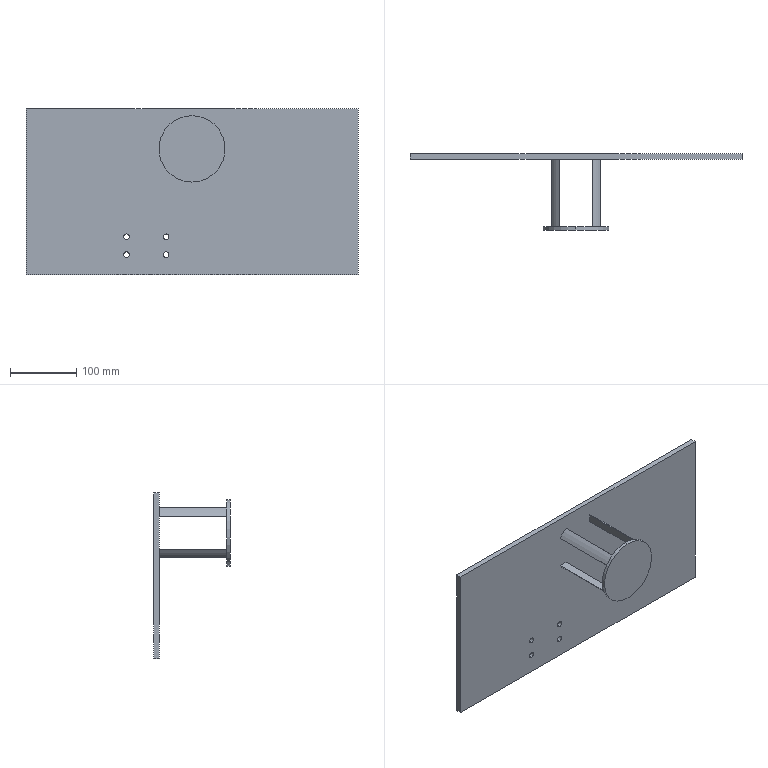Part | SolidWorks | features BaseBody 1 | 1 solid | 30 faces | box 500 x 114.889 x 250 mm | volume 1072983 mm3 | plane 16 | cylinder 14 | commonest cylinder face diameters 8.55 x8 90 x4 100 x2
STEP:
#1=CARTESIAN_POINT('',(211.045,8.,61.824));
#2=VERTEX_POINT('',#1);
#3=CARTESIAN_POINT('',(211.045,8.,53.274));
#4=VERTEX_POINT('',#3);
#5=CARTESIAN_POINT('',(211.045,8.,57.549));
#6=DIRECTION('',(0.,-1.,0.));
#7=DIRECTION('',(0.,0.,-1.));
#8=AXIS2_PLACEMENT_3D('',#5,#6,#7);
#9=CIRCLE('',#8,4.275);
#10=EDGE_CURVE('',#2,#4,#9,.T.);
#11=ORIENTED_EDGE('',*,*,#10,.F.);
#12=CARTESIAN_POINT('',(211.045,0.,61.824));
#13=VERTEX_POINT('',#12);
#14=CARTESIAN_POINT('',(211.045,8.,61.824));
#15=DIRECTION('',(0.,-1.,0.));
#16=VECTOR('',#15,1000.);
#17=LINE('',#14,#16);
#18=EDGE_CURVE('',#2,#13,#17,.T.);
#19=ORIENTED_EDGE('',*,*,#18,.T.);
#20=CARTESIAN_POINT('',(211.045,0.,53.274));
#21=VERTEX_POINT('',#20);
#22=CARTESIAN_POINT('',(211.045,0.,57.549));
#23=DIRECTION('',(0.,1.,0.));
#24=DIRECTION('',(0.,0.,-1.));
#25=AXIS2_PLACEMENT_3D('',#22,#23,#24);
#26=CIRCLE('',#25,4.275);
#27=EDGE_CURVE('',#21,#13,#26,.T.);
#28=ORIENTED_EDGE('',*,*,#27,.F.);
#29=CARTESIAN_POINT('',(211.045,8.,53.274));
#30=DIRECTION('',(0.,-1.,0.));
#31=VECTOR('',#30,1000.);
#32=LINE('',#29,#31);
#33=EDGE_CURVE('',#4,#21,#32,.T.);
#34=ORIENTED_EDGE('',*,*,#33,.F.);
#35=EDGE_LOOP('',(#11,#19,#28,#34));
#36=FACE_OUTER_BOUND('',#35,.T.);
#37=CARTESIAN_POINT('',(211.045,8.,57.549));
#38=DIRECTION('',(0.,-1.,0.));
#39=DIRECTION('',(0.,0.,-1.));
#40=AXIS2_PLACEMENT_3D('',#37,#38,#39);
#41=CYLINDRICAL_SURFACE('',#40,4.275);
#42=ADVANCED_FACE('',(#36),#41,.F.);
#43=CARTESIAN_POINT('',(211.045,8.,34.804));
#44=VERTEX_POINT('',#43);
#45=CARTESIAN_POINT('',(211.045,8.,26.254));
#46=VERTEX_POINT('',#45);
#47=CARTESIAN_POINT('',(211.045,8.,30.529));
#48=DIRECTION('',(0.,-1.,0.));
#49=DIRECTION('',(0.,0.,-1.));
#50=AXIS2_PLACEMENT_3D('',#47,#48,#49);
#51=CIRCLE('',#50,4.275);
#52=EDGE_CURVE('',#44,#46,#51,.T.);
#53=ORIENTED_EDGE('',*,*,#52,.F.);
#54=CARTESIAN_POINT('',(211.045,0.,34.804));
#55=VERTEX_POINT('',#54);
#56=CARTESIAN_POINT('',(211.045,8.,34.804));
#57=DIRECTION('',(0.,-1.,0.));
#58=VECTOR('',#57,1000.);
#59=LINE('',#56,#58);
#60=EDGE_CURVE('',#44,#55,#59,.T.);
#61=ORIENTED_EDGE('',*,*,#60,.T.);
#62=CARTESIAN_POINT('',(211.045,0.,26.254));
#63=VERTEX_POINT('',#62);
#64=CARTESIAN_POINT('',(211.045,0.,30.529));
#65=DIRECTION('',(0.,1.,0.));
#66=DIRECTION('',(0.,0.,-1.));
#67=AXIS2_PLACEMENT_3D('',#64,#65,#66);
#68=CIRCLE('',#67,4.275);
#69=EDGE_CURVE('',#63,#55,#68,.T.);
#70=ORIENTED_EDGE('',*,*,#69,.F.);
#71=CARTESIAN_POINT('',(211.045,8.,26.254));
#72=DIRECTION('',(0.,-1.,0.));
#73=VECTOR('',#72,1000.);
#74=LINE('',#71,#73);
#75=EDGE_CURVE('',#46,#63,#74,.T.);
#76=ORIENTED_EDGE('',*,*,#75,.F.);
#77=EDGE_LOOP('',(#53,#61,#70,#76));
#78=FACE_OUTER_BOUND('',#77,.T.);
#79=CARTESIAN_POINT('',(211.045,8.,30.529));
#80=DIRECTION('',(0.,-1.,0.));
#81=DIRECTION('',(0.,0.,-1.));
#82=AXIS2_PLACEMENT_3D('',#79,#80,#81);
#83=CYLINDRICAL_SURFACE('',#82,4.275);
#84=ADVANCED_FACE('',(#78),#83,.F.);
#85=CARTESIAN_POINT('',(151.435,8.,34.804));
#86=VERTEX_POINT('',#85);
#87=CARTESIAN_POINT('',(151.435,8.,26.254));
#88=VERTEX_POINT('',#87);
#89=CARTESIAN_POINT('',(151.435,8.,30.529));
#90=DIRECTION('',(0.,-1.,0.));
#91=DIRECTION('',(0.,0.,-1.));
#92=AXIS2_PLACEMENT_3D('',#89,#90,#91);
#93=CIRCLE('',#92,4.275);
#94=EDGE_CURVE('',#86,#88,#93,.T.);
#95=ORIENTED_EDGE('',*,*,#94,.F.);
#96=CARTESIAN_POINT('',(151.435,0.,34.804));
#97=VERTEX_POINT('',#96);
#98=CARTESIAN_POINT('',(151.435,8.,34.804));
#99=DIRECTION('',(0.,-1.,0.));
#100=VECTOR('',#99,1000.);
#101=LINE('',#98,#100);
#102=EDGE_CURVE('',#86,#97,#101,.T.);
#103=ORIENTED_EDGE('',*,*,#102,.T.);
#104=CARTESIAN_POINT('',(151.435,0.,26.254));
#105=VERTEX_POINT('',#104);
#106=CARTESIAN_POINT('',(151.435,0.,30.529));
#107=DIRECTION('',(0.,1.,0.));
#108=DIRECTION('',(0.,0.,-1.));
#109=AXIS2_PLACEMENT_3D('',#106,#107,#108);
#110=CIRCLE('',#109,4.275);
#111=EDGE_CURVE('',#105,#97,#110,.T.);
#112=ORIENTED_EDGE('',*,*,#111,.F.);
#113=CARTESIAN_POINT('',(151.435,8.,26.254));
#114=DIRECTION('',(0.,-1.,0.));
#115=VECTOR('',#114,1000.);
#116=LINE('',#113,#115);
#117=EDGE_CURVE('',#88,#105,#116,.T.);
#118=ORIENTED_EDGE('',*,*,#117,.F.);
#119=EDGE_LOOP('',(#95,#103,#112,#118));
#120=FACE_OUTER_BOUND('',#119,.T.);
#121=CARTESIAN_POINT('',(151.435,8.,30.529));
#122=DIRECTION('',(0.,-1.,0.));
#123=DIRECTION('',(0.,0.,-1.));
#124=AXIS2_PLACEMENT_3D('',#121,#122,#123);
#125=CYLINDRICAL_SURFACE('',#124,4.275);
#126=ADVANCED_FACE('',(#120),#125,.F.);
#127=CARTESIAN_POINT('',(151.435,8.,61.824));
#128=VERTEX_POINT('',#127);
#129=CARTESIAN_POINT('',(151.435,8.,53.274));
#130=VERTEX_POINT('',#129);
#131=CARTESIAN_POINT('',(151.435,8.,57.549));
#132=DIRECTION('',(0.,-1.,0.));
#133=DIRECTION('',(0.,0.,-1.));
#134=AXIS2_PLACEMENT_3D('',#131,#132,#133);
#135=CIRCLE('',#134,4.275);
#136=EDGE_CURVE('',#128,#130,#135,.T.);
#137=ORIENTED_EDGE('',*,*,#136,.F.);
#138=CARTESIAN_POINT('',(151.435,0.,61.824));
#139=VERTEX_POINT('',#138);
#140=CARTESIAN_POINT('',(151.435,8.,61.824));
#141=DIRECTION('',(0.,-1.,0.));
#142=VECTOR('',#141,1000.);
#143=LINE('',#140,#142);
#144=EDGE_CURVE('',#128,#139,#143,.T.);
#145=ORIENTED_EDGE('',*,*,#144,.T.);
#146=CARTESIAN_POINT('',(151.435,0.,53.274));
#147=VERTEX_POINT('',#146);
#148=CARTESIAN_POINT('',(151.435,0.,57.549));
#149=DIRECTION('',(0.,1.,0.));
#150=DIRECTION('',(0.,0.,-1.));
#151=AXIS2_PLACEMENT_3D('',#148,#149,#150);
#152=CIRCLE('',#151,4.275);
#153=EDGE_CURVE('',#147,#139,#152,.T.);
#154=ORIENTED_EDGE('',*,*,#153,.F.);
#155=CARTESIAN_POINT('',(151.435,8.,53.274));
#156=DIRECTION('',(0.,-1.,0.));
#157=VECTOR('',#156,1000.);
#158=LINE('',#155,#157);
#159=EDGE_CURVE('',#130,#147,#158,.T.);
#160=ORIENTED_EDGE('',*,*,#159,.F.);
#161=EDGE_LOOP('',(#137,#145,#154,#160));
#162=FACE_OUTER_BOUND('',#161,.T.);
#163=CARTESIAN_POINT('',(151.435,8.,57.549));
#164=DIRECTION('',(0.,-1.,0.));
#165=DIRECTION('',(0.,0.,-1.));
#166=AXIS2_PLACEMENT_3D('',#163,#164,#165);
#167=CYLINDRICAL_SURFACE('',#166,4.275);
#168=ADVANCED_FACE('',(#162),#167,.F.);
#169=CARTESIAN_POINT('',(250.,-106.889,240.));
#170=VERTEX_POINT('',#169);
#171=CARTESIAN_POINT('',(250.,-106.889,140.));
#172=VERTEX_POINT('',#171);
#173=CARTESIAN_POINT('',(250.,-106.889,190.));
#174=DIRECTION('',(0.,1.,0.));
#175=DIRECTION('',(0.,0.,1.));
#176=AXIS2_PLACEMENT_3D('',#173,#174,#175);
#177=CIRCLE('',#176,50.);
#178=EDGE_CURVE('',#170,#172,#177,.T.);
#179=ORIENTED_EDGE('',*,*,#178,.T.);
#180=CARTESIAN_POINT('',(250.,-101.889,140.));
#181=VERTEX_POINT('',#180);
#182=CARTESIAN_POINT('',(250.,-106.889,140.));
#183=DIRECTION('',(0.,1.,0.));
#184=VECTOR('',#183,1000.);
#185=LINE('',#182,#184);
#186=EDGE_CURVE('',#172,#181,#185,.T.);
#187=ORIENTED_EDGE('',*,*,#186,.T.);
#188=CARTESIAN_POINT('',(250.,-101.889,240.));
#189=VERTEX_POINT('',#188);
#190=CARTESIAN_POINT('',(250.,-101.889,190.));
#191=DIRECTION('',(0.,-1.,0.));
#192=DIRECTION('',(0.,0.,1.));
#193=AXIS2_PLACEMENT_3D('',#190,#191,#192);
#194=CIRCLE('',#193,50.);
#195=EDGE_CURVE('',#181,#189,#194,.T.);
#196=ORIENTED_EDGE('',*,*,#195,.T.);
#197=CARTESIAN_POINT('',(250.,-106.889,240.));
#198=DIRECTION('',(0.,1.,0.));
#199=VECTOR('',#198,1000.);
#200=LINE('',#197,#199);
#201=EDGE_CURVE('',#170,#189,#200,.T.);
#202=ORIENTED_EDGE('',*,*,#201,.F.);
#203=EDGE_LOOP('',(#179,#187,#196,#202));
#204=FACE_OUTER_BOUND('',#203,.T.);
#205=CARTESIAN_POINT('',(250.,-106.889,190.));
#206=DIRECTION('',(0.,1.,0.));
#207=DIRECTION('',(0.,0.,1.));
#208=AXIS2_PLACEMENT_3D('',#205,#206,#207);
#209=CYLINDRICAL_SURFACE('',#208,50.);
#210=ADVANCED_FACE('',(#204),#209,.T.);
#211=CARTESIAN_POINT('',(211.045,8.,57.549));
#212=DIRECTION('',(0.,-1.,0.));
#213=DIRECTION('',(0.,0.,-1.));
#214=AXIS2_PLACEMENT_3D('',#211,#212,#213);
#215=CIRCLE('',#214,4.275);
#216=EDGE_CURVE('',#4,#2,#215,.T.);
#217=ORIENTED_EDGE('',*,*,#216,.T.);
#218=ORIENTED_EDGE('',*,*,#10,.T.);
#219=EDGE_LOOP('',(#217,#218));
#220=FACE_BOUND('',#219,.T.);
#221=CARTESIAN_POINT('',(211.045,8.,30.529));
#222=DIRECTION('',(0.,-1.,0.));
#223=DIRECTION('',(0.,0.,-1.));
#224=AXIS2_PLACEMENT_3D('',#221,#222,#223);
#225=CIRCLE('',#224,4.275);
#226=EDGE_CURVE('',#46,#44,#225,.T.);
#227=ORIENTED_EDGE('',*,*,#226,.T.);
#228=ORIENTED_EDGE('',*,*,#52,.T.);
#229=EDGE_LOOP('',(#227,#228));
#230=FACE_BOUND('',#229,.T.);
#231=CARTESIAN_POINT('',(500.,8.,250.));
#232=VERTEX_POINT('',#231);
#233=CARTESIAN_POINT('',(500.,8.,0.));
#234=VERTEX_POINT('',#233);
#235=CARTESIAN_POINT('',(500.,8.,0.));
#236=DIRECTION('',(0.,0.,-1.));
#237=VECTOR('',#236,1000.);
#238=LINE('',#235,#237);
#239=EDGE_CURVE('',#232,#234,#238,.T.);
#240=ORIENTED_EDGE('',*,*,#239,.T.);
#241=CARTESIAN_POINT('',(0.,8.,0.));
#242=VERTEX_POINT('',#241);
#243=CARTESIAN_POINT('',(0.,8.,0.));
#244=DIRECTION('',(-1.,0.,0.));
#245=VECTOR('',#244,1000.);
#246=LINE('',#243,#245);
#247=EDGE_CURVE('',#234,#242,#246,.T.);
#248=ORIENTED_EDGE('',*,*,#247,.T.);
#249=CARTESIAN_POINT('',(0.,8.,250.));
#250=VERTEX_POINT('',#249);
#251=CARTESIAN_POINT('',(0.,8.,0.));
#252=DIRECTION('',(0.,0.,1.));
#253=VECTOR('',#252,1000.);
#254=LINE('',#251,#253);
#255=EDGE_CURVE('',#242,#250,#254,.T.);
#256=ORIENTED_EDGE('',*,*,#255,.T.);
#257=CARTESIAN_POINT('',(0.,8.,250.));
#258=DIRECTION('',(1.,0.,0.));
#259=VECTOR('',#258,1000.);
#260=LINE('',#257,#259);
#261=EDGE_CURVE('',#250,#232,#260,.T.);
#262=ORIENTED_EDGE('',*,*,#261,.T.);
#263=EDGE_LOOP('',(#240,#248,#256,#262));
#264=FACE_OUTER_BOUND('',#263,.T.);
#265=CARTESIAN_POINT('',(151.435,8.,30.529));
#266=DIRECTION('',(0.,-1.,0.));
#267=DIRECTION('',(0.,0.,-1.));
#268=AXIS2_PLACEMENT_3D('',#265,#266,#267);
#269=CIRCLE('',#268,4.275);
#270=EDGE_CURVE('',#88,#86,#269,.T.);
#271=ORIENTED_EDGE('',*,*,#270,.T.);
#272=ORIENTED_EDGE('',*,*,#94,.T.);
#273=EDGE_LOOP('',(#271,#272));
#274=FACE_BOUND('',#273,.T.);
#275=CARTESIAN_POINT('',(151.435,8.,57.549));
#276=DIRECTION('',(0.,-1.,0.));
#277=DIRECTION('',(0.,0.,-1.));
#278=AXIS2_PLACEMENT_3D('',#275,#276,#277);
#279=CIRCLE('',#278,4.275);
#280=EDGE_CURVE('',#130,#128,#279,.T.);
#281=ORIENTED_EDGE('',*,*,#280,.T.);
#282=ORIENTED_EDGE('',*,*,#136,.T.);
#283=EDGE_LOOP('',(#281,#282));
#284=FACE_BOUND('',#283,.T.);
#285=CARTESIAN_POINT('',(0.,8.,0.));
#286=DIRECTION('',(0.,1.,0.));
#287=DIRECTION('',(0.,0.,1.));
#288=AXIS2_PLACEMENT_3D('',#285,#286,#287);
#289=PLANE('',#288);
#290=ADVANCED_FACE('',(#220,#230,#264,#274,#284),#289,.T.);
#291=ORIENTED_EDGE('',*,*,#18,.F.);
#292=ORIENTED_EDGE('',*,*,#216,.F.);
#293=ORIENTED_EDGE('',*,*,#33,.T.);
#294=CARTESIAN_POINT('',(211.045,0.,57.549));
#295=DIRECTION('',(0.,1.,0.));
#296=DIRECTION('',(0.,0.,-1.));
#297=AXIS2_PLACEMENT_3D('',#294,#295,#296);
#298=CIRCLE('',#297,4.275);
#299=EDGE_CURVE('',#13,#21,#298,.T.);
#300=ORIENTED_EDGE('',*,*,#299,.F.);
#301=EDGE_LOOP('',(#291,#292,#293,#300));
#302=FACE_OUTER_BOUND('',#301,.T.);
#303=CARTESIAN_POINT('',(211.045,8.,57.549));
#304=DIRECTION('',(0.,-1.,0.));
#305=DIRECTION('',(0.,0.,-1.));
#306=AXIS2_PLACEMENT_3D('',#303,#304,#305);
#307=CYLINDRICAL_SURFACE('',#306,4.275);
#308=ADVANCED_FACE('',(#302),#307,.F.);
#309=ORIENTED_EDGE('',*,*,#60,.F.);
#310=ORIENTED_EDGE('',*,*,#226,.F.);
#311=ORIENTED_EDGE('',*,*,#75,.T.);
#312=CARTESIAN_POINT('',(211.045,0.,30.529));
#313=DIRECTION('',(0.,1.,0.));
#314=DIRECTION('',(0.,0.,-1.));
#315=AXIS2_PLACEMENT_3D('',#312,#313,#314);
#316=CIRCLE('',#315,4.275);
#317=EDGE_CURVE('',#55,#63,#316,.T.);
#318=ORIENTED_EDGE('',*,*,#317,.F.);
#319=EDGE_LOOP('',(#309,#310,#311,#318));
#320=FACE_OUTER_BOUND('',#319,.T.);
#321=CARTESIAN_POINT('',(211.045,8.,30.529));
#322=DIRECTION('',(0.,-1.,0.));
#323=DIRECTION('',(0.,0.,-1.));
#324=AXIS2_PLACEMENT_3D('',#321,#322,#323);
#325=CYLINDRICAL_SURFACE('',#324,4.275);
#326=ADVANCED_FACE('',(#320),#325,.F.);
#327=CARTESIAN_POINT('',(0.,0.,0.));
#328=VERTEX_POINT('',#327);
#329=CARTESIAN_POINT('',(0.,8.,0.));
#330=DIRECTION('',(0.,-1.,0.));
#331=VECTOR('',#330,1000.);
#332=LINE('',#329,#331);
#333=EDGE_CURVE('',#242,#328,#332,.T.);
#334=ORIENTED_EDGE('',*,*,#333,.F.);
#335=ORIENTED_EDGE('',*,*,#247,.F.);
#336=CARTESIAN_POINT('',(500.,0.,0.));
#337=VERTEX_POINT('',#336);
#338=CARTESIAN_POINT('',(500.,8.,0.));
#339=DIRECTION('',(0.,1.,0.));
#340=VECTOR('',#339,1000.);
#341=LINE('',#338,#340);
#342=EDGE_CURVE('',#337,#234,#341,.T.);
#343=ORIENTED_EDGE('',*,*,#342,.F.);
#344=CARTESIAN_POINT('',(0.,0.,0.));
#345=DIRECTION('',(1.,0.,0.));
#346=VECTOR('',#345,1000.);
#347=LINE('',#344,#346);
#348=EDGE_CURVE('',#328,#337,#347,.T.);
#349=ORIENTED_EDGE('',*,*,#348,.F.);
#350=EDGE_LOOP('',(#334,#335,#343,#349));
#351=FACE_OUTER_BOUND('',#350,.T.);
#352=CARTESIAN_POINT('',(0.,8.,0.));
#353=DIRECTION('',(0.,0.,1.));
#354=DIRECTION('',(1.,0.,0.));
#355=AXIS2_PLACEMENT_3D('',#352,#353,#354);
#356=PLANE('',#355);
#357=ADVANCED_FACE('',(#351),#356,.F.);
#358=ORIENTED_EDGE('',*,*,#342,.T.);
#359=ORIENTED_EDGE('',*,*,#239,.F.);
#360=CARTESIAN_POINT('',(500.,0.,250.));
#361=VERTEX_POINT('',#360);
#362=CARTESIAN_POINT('',(500.,8.,250.));
#363=DIRECTION('',(0.,1.,0.));
#364=VECTOR('',#363,1000.);
#365=LINE('',#362,#364);
#366=EDGE_CURVE('',#361,#232,#365,.T.);
#367=ORIENTED_EDGE('',*,*,#366,.F.);
#368=CARTESIAN_POINT('',(500.,0.,0.));
#369=DIRECTION('',(0.,0.,1.));
#370=VECTOR('',#369,1000.);
#371=LINE('',#368,#370);
#372=EDGE_CURVE('',#337,#361,#371,.T.);
#373=ORIENTED_EDGE('',*,*,#372,.F.);
#374=EDGE_LOOP('',(#358,#359,#367,#373));
#375=FACE_OUTER_BOUND('',#374,.T.);
#376=CARTESIAN_POINT('',(500.,8.,0.));
#377=DIRECTION('',(-1.,0.,0.));
#378=DIRECTION('',(0.,0.,1.));
#379=AXIS2_PLACEMENT_3D('',#376,#377,#378);
#380=PLANE('',#379);
#381=ADVANCED_FACE('',(#375),#380,.F.);
#382=ORIENTED_EDGE('',*,*,#366,.T.);
#383=ORIENTED_EDGE('',*,*,#261,.F.);
#384=CARTESIAN_POINT('',(0.,0.,250.));
#385=VERTEX_POINT('',#384);
#386=CARTESIAN_POINT('',(0.,8.,250.));
#387=DIRECTION('',(0.,1.,0.));
#388=VECTOR('',#387,1000.);
#389=LINE('',#386,#388);
#390=EDGE_CURVE('',#385,#250,#389,.T.);
#391=ORIENTED_EDGE('',*,*,#390,.F.);
#392=CARTESIAN_POINT('',(0.,0.,250.));
#393=DIRECTION('',(-1.,0.,0.));
#394=VECTOR('',#393,1000.);
#395=LINE('',#392,#394);
#396=EDGE_CURVE('',#361,#385,#395,.T.);
#397=ORIENTED_EDGE('',*,*,#396,.F.);
#398=EDGE_LOOP('',(#382,#383,#391,#397));
#399=FACE_OUTER_BOUND('',#398,.T.);
#400=CARTESIAN_POINT('',(0.,8.,250.));
#401=DIRECTION('',(0.,0.,-1.));
#402=DIRECTION('',(-1.,0.,0.));
#403=AXIS2_PLACEMENT_3D('',#400,#401,#402);
#404=PLANE('',#403);
#405=ADVANCED_FACE('',(#399),#404,.F.);
#406=ORIENTED_EDGE('',*,*,#390,.T.);
#407=ORIENTED_EDGE('',*,*,#255,.F.);
#408=ORIENTED_EDGE('',*,*,#333,.T.);
#409=CARTESIAN_POINT('',(0.,0.,0.));
#410=DIRECTION('',(0.,0.,-1.));
#411=VECTOR('',#410,1000.);
#412=LINE('',#409,#411);
#413=EDGE_CURVE('',#385,#328,#412,.T.);
#414=ORIENTED_EDGE('',*,*,#413,.F.);
#415=EDGE_LOOP('',(#406,#407,#408,#414));
#416=FACE_OUTER_BOUND('',#415,.T.);
#417=CARTESIAN_POINT('',(0.,8.,0.));
#418=DIRECTION('',(1.,0.,0.));
#419=DIRECTION('',(0.,0.,-1.));
#420=AXIS2_PLACEMENT_3D('',#417,#418,#419);
#421=PLANE('',#420);
#422=ADVANCED_FACE('',(#416),#421,.F.);
#423=ORIENTED_EDGE('',*,*,#102,.F.);
#424=ORIENTED_EDGE('',*,*,#270,.F.);
#425=ORIENTED_EDGE('',*,*,#117,.T.);
#426=CARTESIAN_POINT('',(151.435,0.,30.529));
#427=DIRECTION('',(0.,1.,0.));
#428=DIRECTION('',(0.,0.,-1.));
#429=AXIS2_PLACEMENT_3D('',#426,#427,#428);
#430=CIRCLE('',#429,4.275);
#431=EDGE_CURVE('',#97,#105,#430,.T.);
#432=ORIENTED_EDGE('',*,*,#431,.F.);
#433=EDGE_LOOP('',(#423,#424,#425,#432));
#434=FACE_OUTER_BOUND('',#433,.T.);
#435=CARTESIAN_POINT('',(151.435,8.,30.529));
#436=DIRECTION('',(0.,-1.,0.));
#437=DIRECTION('',(0.,0.,-1.));
#438=AXIS2_PLACEMENT_3D('',#435,#436,#437);
#439=CYLINDRICAL_SURFACE('',#438,4.275);
#440=ADVANCED_FACE('',(#434),#439,.F.);
#441=ORIENTED_EDGE('',*,*,#144,.F.);
#442=ORIENTED_EDGE('',*,*,#280,.F.);
#443=ORIENTED_EDGE('',*,*,#159,.T.);
#444=CARTESIAN_POINT('',(151.435,0.,57.549));
#445=DIRECTION('',(0.,1.,0.));
#446=DIRECTION('',(0.,0.,-1.));
#447=AXIS2_PLACEMENT_3D('',#444,#445,#446);
#448=CIRCLE('',#447,4.275);
#449=EDGE_CURVE('',#139,#147,#448,.T.);
#450=ORIENTED_EDGE('',*,*,#449,.F.);
#451=EDGE_LOOP('',(#441,#442,#443,#450));
#452=FACE_OUTER_BOUND('',#451,.T.);
#453=CARTESIAN_POINT('',(151.435,8.,57.549));
#454=DIRECTION('',(0.,-1.,0.));
#455=DIRECTION('',(0.,0.,-1.));
#456=AXIS2_PLACEMENT_3D('',#453,#454,#455);
#457=CYLINDRICAL_SURFACE('',#456,4.275);
#458=ADVANCED_FACE('',(#452),#457,.F.);
#459=CARTESIAN_POINT('',(225.,0.,165.));
#460=VERTEX_POINT('',#459);
#461=CARTESIAN_POINT('',(212.583,0.,165.));
#462=VERTEX_POINT('',#461);
#463=CARTESIAN_POINT('',(0.,0.,165.));
#464=DIRECTION('',(-1.,0.,0.));
#465=VECTOR('',#464,1000.);
#466=LINE('',#463,#465);
#467=EDGE_CURVE('',#460,#462,#466,.T.);
#468=ORIENTED_EDGE('',*,*,#467,.F.);
#469=CARTESIAN_POINT('',(225.,0.,152.583));
#470=VERTEX_POINT('',#469);
#471=CARTESIAN_POINT('',(225.,0.,0.));
#472=DIRECTION('',(0.,0.,1.));
#473=VECTOR('',#472,1000.);
#474=LINE('',#471,#473);
#475=EDGE_CURVE('',#470,#460,#474,.T.);
#476=ORIENTED_EDGE('',*,*,#475,.F.);
#477=CARTESIAN_POINT('',(250.,0.,190.));
#478=DIRECTION('',(0.,-1.,0.));
#479=DIRECTION('',(0.,0.,1.));
#480=AXIS2_PLACEMENT_3D('',#477,#478,#479);
#481=CIRCLE('',#480,45.);
#482=EDGE_CURVE('',#462,#470,#481,.T.);
#483=ORIENTED_EDGE('',*,*,#482,.F.);
#484=EDGE_LOOP('',(#468,#476,#483));
#485=FACE_BOUND('',#484,.T.);
#486=CARTESIAN_POINT('',(225.,0.,215.));
#487=VERTEX_POINT('',#486);
#488=CARTESIAN_POINT('',(225.,0.,227.417));
#489=VERTEX_POINT('',#488);
#490=CARTESIAN_POINT('',(225.,0.,0.));
#491=DIRECTION('',(0.,0.,1.));
#492=VECTOR('',#491,1000.);
#493=LINE('',#490,#492);
#494=EDGE_CURVE('',#487,#489,#493,.T.);
#495=ORIENTED_EDGE('',*,*,#494,.F.);
#496=CARTESIAN_POINT('',(212.583,0.,215.));
#497=VERTEX_POINT('',#496);
#498=CARTESIAN_POINT('',(0.,0.,215.));
#499=DIRECTION('',(1.,0.,0.));
#500=VECTOR('',#499,1000.);
#501=LINE('',#498,#500);
#502=EDGE_CURVE('',#497,#487,#501,.T.);
#503=ORIENTED_EDGE('',*,*,#502,.F.);
#504=CARTESIAN_POINT('',(250.,0.,190.));
#505=DIRECTION('',(0.,-1.,0.));
#506=DIRECTION('',(0.,0.,1.));
#507=AXIS2_PLACEMENT_3D('',#504,#505,#506);
#508=CIRCLE('',#507,45.);
#509=EDGE_CURVE('',#489,#497,#508,.T.);
#510=ORIENTED_EDGE('',*,*,#509,.F.);
#511=EDGE_LOOP('',(#495,#503,#510));
#512=FACE_BOUND('',#511,.T.);
#513=ORIENTED_EDGE('',*,*,#27,.T.);
#514=ORIENTED_EDGE('',*,*,#299,.T.);
#515=EDGE_LOOP('',(#513,#514));
#516=FACE_BOUND('',#515,.T.);
#517=ORIENTED_EDGE('',*,*,#153,.T.);
#518=ORIENTED_EDGE('',*,*,#449,.T.);
#519=EDGE_LOOP('',(#517,#518));
#520=FACE_BOUND('',#519,.T.);
#521=ORIENTED_EDGE('',*,*,#69,.T.);
#522=ORIENTED_EDGE('',*,*,#317,.T.);
#523=EDGE_LOOP('',(#521,#522));
#524=FACE_BOUND('',#523,.T.);
#525=ORIENTED_EDGE('',*,*,#111,.T.);
#526=ORIENTED_EDGE('',*,*,#431,.T.);
#527=EDGE_LOOP('',(#525,#526));
#528=FACE_BOUND('',#527,.T.);
#529=ORIENTED_EDGE('',*,*,#348,.T.);
#530=ORIENTED_EDGE('',*,*,#372,.T.);
#531=ORIENTED_EDGE('',*,*,#396,.T.);
#532=ORIENTED_EDGE('',*,*,#413,.T.);
#533=EDGE_LOOP('',(#529,#530,#531,#532));
#534=FACE_OUTER_BOUND('',#533,.T.);
#535=CARTESIAN_POINT('',(275.,0.,227.417));
#536=VERTEX_POINT('',#535);
#537=CARTESIAN_POINT('',(275.,0.,215.));
#538=VERTEX_POINT('',#537);
#539=CARTESIAN_POINT('',(275.,0.,0.));
#540=DIRECTION('',(0.,0.,-1.));
#541=VECTOR('',#540,1000.);
#542=LINE('',#539,#541);
#543=EDGE_CURVE('',#536,#538,#542,.T.);
#544=ORIENTED_EDGE('',*,*,#543,.F.);
#545=CARTESIAN_POINT('',(287.417,0.,215.));
#546=VERTEX_POINT('',#545);
#547=CARTESIAN_POINT('',(250.,0.,190.));
#548=DIRECTION('',(0.,-1.,0.));
#549=DIRECTION('',(0.,0.,1.));
#550=AXIS2_PLACEMENT_3D('',#547,#548,#549);
#551=CIRCLE('',#550,45.);
#552=EDGE_CURVE('',#546,#536,#551,.T.);
#553=ORIENTED_EDGE('',*,*,#552,.F.);
#554=CARTESIAN_POINT('',(0.,0.,215.));
#555=DIRECTION('',(1.,0.,0.));
#556=VECTOR('',#555,1000.);
#557=LINE('',#554,#556);
#558=EDGE_CURVE('',#538,#546,#557,.T.);
#559=ORIENTED_EDGE('',*,*,#558,.F.);
#560=EDGE_LOOP('',(#544,#553,#559));
#561=FACE_BOUND('',#560,.T.);
#562=CARTESIAN_POINT('',(275.,0.,165.));
#563=VERTEX_POINT('',#562);
#564=CARTESIAN_POINT('',(275.,0.,152.583));
#565=VERTEX_POINT('',#564);
#566=CARTESIAN_POINT('',(275.,0.,0.));
#567=DIRECTION('',(0.,0.,-1.));
#568=VECTOR('',#567,1000.);
#569=LINE('',#566,#568);
#570=EDGE_CURVE('',#563,#565,#569,.T.);
#571=ORIENTED_EDGE('',*,*,#570,.F.);
#572=CARTESIAN_POINT('',(287.417,0.,165.));
#573=VERTEX_POINT('',#572);
#574=CARTESIAN_POINT('',(0.,0.,165.));
#575=DIRECTION('',(-1.,0.,0.));
#576=VECTOR('',#575,1000.);
#577=LINE('',#574,#576);
#578=EDGE_CURVE('',#573,#563,#577,.T.);
#579=ORIENTED_EDGE('',*,*,#578,.F.);
#580=CARTESIAN_POINT('',(250.,0.,190.));
#581=DIRECTION('',(0.,-1.,0.));
#582=DIRECTION('',(0.,0.,1.));
#583=AXIS2_PLACEMENT_3D('',#580,#581,#582);
#584=CIRCLE('',#583,45.);
#585=EDGE_CURVE('',#565,#573,#584,.T.);
#586=ORIENTED_EDGE('',*,*,#585,.F.);
#587=EDGE_LOOP('',(#571,#579,#586));
#588=FACE_BOUND('',#587,.T.);
#589=CARTESIAN_POINT('',(0.,0.,0.));
#590=DIRECTION('',(0.,1.,0.));
#591=DIRECTION('',(0.,0.,1.));
#592=AXIS2_PLACEMENT_3D('',#589,#590,#591);
#593=PLANE('',#592);
#594=ADVANCED_FACE('',(#485,#512,#516,#520,#524,#528,#534,#561,#588),#593,.F.);
#595=CARTESIAN_POINT('',(225.,-101.889,152.583));
#596=VERTEX_POINT('',#595);
#597=CARTESIAN_POINT('',(212.583,-101.889,165.));
#598=VERTEX_POINT('',#597);
#599=CARTESIAN_POINT('',(250.,-101.889,190.));
#600=DIRECTION('',(0.,1.,0.));
#601=DIRECTION('',(0.,0.,1.));
#602=AXIS2_PLACEMENT_3D('',#599,#600,#601);
#603=CIRCLE('',#602,45.);
#604=EDGE_CURVE('',#596,#598,#603,.T.);
#605=ORIENTED_EDGE('',*,*,#604,.T.);
#606=CARTESIAN_POINT('',(212.583,-101.889,165.));
#607=DIRECTION('',(0.,1.,0.));
#608=VECTOR('',#607,1000.);
#609=LINE('',#606,#608);
#610=EDGE_CURVE('',#598,#462,#609,.T.);
#611=ORIENTED_EDGE('',*,*,#610,.T.);
#612=ORIENTED_EDGE('',*,*,#482,.T.);
#613=CARTESIAN_POINT('',(225.,-101.889,152.583));
#614=DIRECTION('',(0.,-1.,0.));
#615=VECTOR('',#614,1000.);
#616=LINE('',#613,#615);
#617=EDGE_CURVE('',#470,#596,#616,.T.);
#618=ORIENTED_EDGE('',*,*,#617,.T.);
#619=EDGE_LOOP('',(#605,#611,#612,#618));
#620=FACE_OUTER_BOUND('',#619,.T.);
#621=CARTESIAN_POINT('',(250.,-101.889,190.));
#622=DIRECTION('',(0.,1.,0.));
#623=DIRECTION('',(0.,0.,1.));
#624=AXIS2_PLACEMENT_3D('',#621,#622,#623);
#625=CYLINDRICAL_SURFACE('',#624,45.);
#626=ADVANCED_FACE('',(#620),#625,.T.);
#627=ORIENTED_EDGE('',*,*,#610,.F.);
#628=CARTESIAN_POINT('',(225.,-101.889,165.));
#629=VERTEX_POINT('',#628);
#630=CARTESIAN_POINT('',(225.,-101.889,165.));
#631=DIRECTION('',(-1.,0.,0.));
#632=VECTOR('',#631,1000.);
#633=LINE('',#630,#632);
#634=EDGE_CURVE('',#629,#598,#633,.T.);
#635=ORIENTED_EDGE('',*,*,#634,.F.);
#636=CARTESIAN_POINT('',(225.,-101.889,165.));
#637=DIRECTION('',(0.,-1.,0.));
#638=VECTOR('',#637,1000.);
#639=LINE('',#636,#638);
#640=EDGE_CURVE('',#460,#629,#639,.T.);
#641=ORIENTED_EDGE('',*,*,#640,.F.);
#642=ORIENTED_EDGE('',*,*,#467,.T.);
#643=EDGE_LOOP('',(#627,#635,#641,#642));
#644=FACE_OUTER_BOUND('',#643,.T.);
#645=CARTESIAN_POINT('',(225.,-101.889,165.));
#646=DIRECTION('',(0.,0.,-1.));
#647=DIRECTION('',(-1.,0.,0.));
#648=AXIS2_PLACEMENT_3D('',#645,#646,#647);
#649=PLANE('',#648);
#650=ADVANCED_FACE('',(#644),#649,.F.);
#651=ORIENTED_EDGE('',*,*,#640,.T.);
#652=CARTESIAN_POINT('',(225.,-101.889,152.583));
#653=DIRECTION('',(0.,0.,1.));
#654=VECTOR('',#653,1000.);
#655=LINE('',#652,#654);
#656=EDGE_CURVE('',#596,#629,#655,.T.);
#657=ORIENTED_EDGE('',*,*,#656,.F.);
#658=ORIENTED_EDGE('',*,*,#617,.F.);
#659=ORIENTED_EDGE('',*,*,#475,.T.);
#660=EDGE_LOOP('',(#651,#657,#658,#659));
#661=FACE_OUTER_BOUND('',#660,.T.);
#662=CARTESIAN_POINT('',(225.,-101.889,152.583));
#663=DIRECTION('',(-1.,0.,0.));
#664=DIRECTION('',(0.,0.,1.));
#665=AXIS2_PLACEMENT_3D('',#662,#663,#664);
#666=PLANE('',#665);
#667=ADVANCED_FACE('',(#661),#666,.F.);
#668=CARTESIAN_POINT('',(212.583,-101.889,215.));
#669=VERTEX_POINT('',#668);
#670=CARTESIAN_POINT('',(225.,-101.889,227.417));
#671=VERTEX_POINT('',#670);
#672=CARTESIAN_POINT('',(250.,-101.889,190.));
#673=DIRECTION('',(0.,1.,0.));
#674=DIRECTION('',(0.,0.,1.));
#675=AXIS2_PLACEMENT_3D('',#672,#673,#674);
#676=CIRCLE('',#675,45.);
#677=EDGE_CURVE('',#669,#671,#676,.T.);
#678=ORIENTED_EDGE('',*,*,#677,.T.);
#679=CARTESIAN_POINT('',(225.,-101.889,227.417));
#680=DIRECTION('',(0.,1.,0.));
#681=VECTOR('',#680,1000.);
#682=LINE('',#679,#681);
#683=EDGE_CURVE('',#671,#489,#682,.T.);
#684=ORIENTED_EDGE('',*,*,#683,.T.);
#685=ORIENTED_EDGE('',*,*,#509,.T.);
#686=CARTESIAN_POINT('',(212.583,-101.889,215.));
#687=DIRECTION('',(0.,-1.,0.));
#688=VECTOR('',#687,1000.);
#689=LINE('',#686,#688);
#690=EDGE_CURVE('',#497,#669,#689,.T.);
#691=ORIENTED_EDGE('',*,*,#690,.T.);
#692=EDGE_LOOP('',(#678,#684,#685,#691));
#693=FACE_OUTER_BOUND('',#692,.T.);
#694=CARTESIAN_POINT('',(250.,-101.889,190.));
#695=DIRECTION('',(0.,1.,0.));
#696=DIRECTION('',(0.,0.,1.));
#697=AXIS2_PLACEMENT_3D('',#694,#695,#696);
#698=CYLINDRICAL_SURFACE('',#697,45.);
#699=ADVANCED_FACE('',(#693),#698,.T.);
#700=ORIENTED_EDGE('',*,*,#683,.F.);
#701=CARTESIAN_POINT('',(225.,-101.889,215.));
#702=VERTEX_POINT('',#701);
#703=CARTESIAN_POINT('',(225.,-101.889,215.));
#704=DIRECTION('',(0.,0.,1.));
#705=VECTOR('',#704,1000.);
#706=LINE('',#703,#705);
#707=EDGE_CURVE('',#702,#671,#706,.T.);
#708=ORIENTED_EDGE('',*,*,#707,.F.);
#709=CARTESIAN_POINT('',(225.,-101.889,215.));
#710=DIRECTION('',(0.,-1.,0.));
#711=VECTOR('',#710,1000.);
#712=LINE('',#709,#711);
#713=EDGE_CURVE('',#487,#702,#712,.T.);
#714=ORIENTED_EDGE('',*,*,#713,.F.);
#715=ORIENTED_EDGE('',*,*,#494,.T.);
#716=EDGE_LOOP('',(#700,#708,#714,#715));
#717=FACE_OUTER_BOUND('',#716,.T.);
#718=CARTESIAN_POINT('',(225.,-101.889,215.));
#719=DIRECTION('',(-1.,0.,0.));
#720=DIRECTION('',(0.,0.,1.));
#721=AXIS2_PLACEMENT_3D('',#718,#719,#720);
#722=PLANE('',#721);
#723=ADVANCED_FACE('',(#717),#722,.F.);
#724=ORIENTED_EDGE('',*,*,#713,.T.);
#725=CARTESIAN_POINT('',(212.583,-101.889,215.));
#726=DIRECTION('',(1.,0.,0.));
#727=VECTOR('',#726,1000.);
#728=LINE('',#725,#727);
#729=EDGE_CURVE('',#669,#702,#728,.T.);
#730=ORIENTED_EDGE('',*,*,#729,.F.);
#731=ORIENTED_EDGE('',*,*,#690,.F.);
#732=ORIENTED_EDGE('',*,*,#502,.T.);
#733=EDGE_LOOP('',(#724,#730,#731,#732));
#734=FACE_OUTER_BOUND('',#733,.T.);
#735=CARTESIAN_POINT('',(212.583,-101.889,215.));
#736=DIRECTION('',(0.,0.,1.));
#737=DIRECTION('',(1.,0.,0.));
#738=AXIS2_PLACEMENT_3D('',#735,#736,#737);
#739=PLANE('',#738);
#740=ADVANCED_FACE('',(#734),#739,.F.);
#741=CARTESIAN_POINT('',(287.417,-101.889,215.));
#742=VERTEX_POINT('',#741);
#743=CARTESIAN_POINT('',(287.417,-101.889,215.));
#744=DIRECTION('',(0.,1.,0.));
#745=VECTOR('',#744,1000.);
#746=LINE('',#743,#745);
#747=EDGE_CURVE('',#742,#546,#746,.T.);
#748=ORIENTED_EDGE('',*,*,#747,.F.);
#749=CARTESIAN_POINT('',(275.,-101.889,215.));
#750=VERTEX_POINT('',#749);
#751=CARTESIAN_POINT('',(275.,-101.889,215.));
#752=DIRECTION('',(1.,0.,0.));
#753=VECTOR('',#752,1000.);
#754=LINE('',#751,#753);
#755=EDGE_CURVE('',#750,#742,#754,.T.);
#756=ORIENTED_EDGE('',*,*,#755,.F.);
#757=CARTESIAN_POINT('',(275.,-101.889,215.));
#758=DIRECTION('',(0.,-1.,0.));
#759=VECTOR('',#758,1000.);
#760=LINE('',#757,#759);
#761=EDGE_CURVE('',#538,#750,#760,.T.);
#762=ORIENTED_EDGE('',*,*,#761,.F.);
#763=ORIENTED_EDGE('',*,*,#558,.T.);
#764=EDGE_LOOP('',(#748,#756,#762,#763));
#765=FACE_OUTER_BOUND('',#764,.T.);
#766=CARTESIAN_POINT('',(275.,-101.889,215.));
#767=DIRECTION('',(0.,0.,1.));
#768=DIRECTION('',(1.,0.,0.));
#769=AXIS2_PLACEMENT_3D('',#766,#767,#768);
#770=PLANE('',#769);
#771=ADVANCED_FACE('',(#765),#770,.F.);
#772=ORIENTED_EDGE('',*,*,#761,.T.);
#773=CARTESIAN_POINT('',(275.,-101.889,227.417));
#774=VERTEX_POINT('',#773);
#775=CARTESIAN_POINT('',(275.,-101.889,227.417));
#776=DIRECTION('',(0.,0.,-1.));
#777=VECTOR('',#776,1000.);
#778=LINE('',#775,#777);
#779=EDGE_CURVE('',#774,#750,#778,.T.);
#780=ORIENTED_EDGE('',*,*,#779,.F.);
#781=CARTESIAN_POINT('',(275.,-101.889,227.417));
#782=DIRECTION('',(0.,-1.,0.));
#783=VECTOR('',#782,1000.);
#784=LINE('',#781,#783);
#785=EDGE_CURVE('',#536,#774,#784,.T.);
#786=ORIENTED_EDGE('',*,*,#785,.F.);
#787=ORIENTED_EDGE('',*,*,#543,.T.);
#788=EDGE_LOOP('',(#772,#780,#786,#787));
#789=FACE_OUTER_BOUND('',#788,.T.);
#790=CARTESIAN_POINT('',(275.,-101.889,227.417));
#791=DIRECTION('',(1.,0.,0.));
#792=DIRECTION('',(0.,0.,-1.));
#793=AXIS2_PLACEMENT_3D('',#790,#791,#792);
#794=PLANE('',#793);
#795=ADVANCED_FACE('',(#789),#794,.F.);
#796=CARTESIAN_POINT('',(250.,-101.889,190.));
#797=DIRECTION('',(0.,1.,0.));
#798=DIRECTION('',(0.,0.,1.));
#799=AXIS2_PLACEMENT_3D('',#796,#797,#798);
#800=CIRCLE('',#799,45.);
#801=EDGE_CURVE('',#774,#742,#800,.T.);
#802=ORIENTED_EDGE('',*,*,#801,.T.);
#803=ORIENTED_EDGE('',*,*,#747,.T.);
#804=ORIENTED_EDGE('',*,*,#552,.T.);
#805=ORIENTED_EDGE('',*,*,#785,.T.);
#806=EDGE_LOOP('',(#802,#803,#804,#805));
#807=FACE_OUTER_BOUND('',#806,.T.);
#808=CARTESIAN_POINT('',(250.,-101.889,190.));
#809=DIRECTION('',(0.,1.,0.));
#810=DIRECTION('',(0.,0.,1.));
#811=AXIS2_PLACEMENT_3D('',#808,#809,#810);
#812=CYLINDRICAL_SURFACE('',#811,45.);
#813=ADVANCED_FACE('',(#807),#812,.T.);
#814=CARTESIAN_POINT('',(287.417,-101.889,165.));
#815=VERTEX_POINT('',#814);
#816=CARTESIAN_POINT('',(275.,-101.889,152.583));
#817=VERTEX_POINT('',#816);
#818=CARTESIAN_POINT('',(250.,-101.889,190.));
#819=DIRECTION('',(0.,1.,0.));
#820=DIRECTION('',(0.,0.,1.));
#821=AXIS2_PLACEMENT_3D('',#818,#819,#820);
#822=CIRCLE('',#821,45.);
#823=EDGE_CURVE('',#815,#817,#822,.T.);
#824=ORIENTED_EDGE('',*,*,#823,.T.);
#825=CARTESIAN_POINT('',(275.,-101.889,152.583));
#826=DIRECTION('',(0.,1.,0.));
#827=VECTOR('',#826,1000.);
#828=LINE('',#825,#827);
#829=EDGE_CURVE('',#817,#565,#828,.T.);
#830=ORIENTED_EDGE('',*,*,#829,.T.);
#831=ORIENTED_EDGE('',*,*,#585,.T.);
#832=CARTESIAN_POINT('',(287.417,-101.889,165.));
#833=DIRECTION('',(0.,-1.,0.));
#834=VECTOR('',#833,1000.);
#835=LINE('',#832,#834);
#836=EDGE_CURVE('',#573,#815,#835,.T.);
#837=ORIENTED_EDGE('',*,*,#836,.T.);
#838=EDGE_LOOP('',(#824,#830,#831,#837));
#839=FACE_OUTER_BOUND('',#838,.T.);
#840=CARTESIAN_POINT('',(250.,-101.889,190.));
#841=DIRECTION('',(0.,1.,0.));
#842=DIRECTION('',(0.,0.,1.));
#843=AXIS2_PLACEMENT_3D('',#840,#841,#842);
#844=CYLINDRICAL_SURFACE('',#843,45.);
#845=ADVANCED_FACE('',(#839),#844,.T.);
#846=ORIENTED_EDGE('',*,*,#829,.F.);
#847=CARTESIAN_POINT('',(275.,-101.889,165.));
#848=VERTEX_POINT('',#847);
#849=CARTESIAN_POINT('',(275.,-101.889,165.));
#850=DIRECTION('',(0.,0.,-1.));
#851=VECTOR('',#850,1000.);
#852=LINE('',#849,#851);
#853=EDGE_CURVE('',#848,#817,#852,.T.);
#854=ORIENTED_EDGE('',*,*,#853,.F.);
#855=CARTESIAN_POINT('',(275.,-101.889,165.));
#856=DIRECTION('',(0.,-1.,0.));
#857=VECTOR('',#856,1000.);
#858=LINE('',#855,#857);
#859=EDGE_CURVE('',#563,#848,#858,.T.);
#860=ORIENTED_EDGE('',*,*,#859,.F.);
#861=ORIENTED_EDGE('',*,*,#570,.T.);
#862=EDGE_LOOP('',(#846,#854,#860,#861));
#863=FACE_OUTER_BOUND('',#862,.T.);
#864=CARTESIAN_POINT('',(275.,-101.889,165.));
#865=DIRECTION('',(1.,0.,0.));
#866=DIRECTION('',(0.,0.,-1.));
#867=AXIS2_PLACEMENT_3D('',#864,#865,#866);
#868=PLANE('',#867);
#869=ADVANCED_FACE('',(#863),#868,.F.);
#870=ORIENTED_EDGE('',*,*,#859,.T.);
#871=CARTESIAN_POINT('',(287.417,-101.889,165.));
#872=DIRECTION('',(-1.,0.,0.));
#873=VECTOR('',#872,1000.);
#874=LINE('',#871,#873);
#875=EDGE_CURVE('',#815,#848,#874,.T.);
#876=ORIENTED_EDGE('',*,*,#875,.F.);
#877=ORIENTED_EDGE('',*,*,#836,.F.);
#878=ORIENTED_EDGE('',*,*,#578,.T.);
#879=EDGE_LOOP('',(#870,#876,#877,#878));
#880=FACE_OUTER_BOUND('',#879,.T.);
#881=CARTESIAN_POINT('',(287.417,-101.889,165.));
#882=DIRECTION('',(0.,0.,-1.));
#883=DIRECTION('',(-1.,0.,0.));
#884=AXIS2_PLACEMENT_3D('',#881,#882,#883);
#885=PLANE('',#884);
#886=ADVANCED_FACE('',(#880),#885,.F.);
#887=ORIENTED_EDGE('',*,*,#755,.T.);
#888=ORIENTED_EDGE('',*,*,#801,.F.);
#889=ORIENTED_EDGE('',*,*,#779,.T.);
#890=EDGE_LOOP('',(#887,#888,#889));
#891=FACE_BOUND('',#890,.T.);
#892=ORIENTED_EDGE('',*,*,#677,.F.);
#893=ORIENTED_EDGE('',*,*,#729,.T.);
#894=ORIENTED_EDGE('',*,*,#707,.T.);
#895=EDGE_LOOP('',(#892,#893,#894));
#896=FACE_BOUND('',#895,.T.);
#897=ORIENTED_EDGE('',*,*,#823,.F.);
#898=ORIENTED_EDGE('',*,*,#875,.T.);
#899=ORIENTED_EDGE('',*,*,#853,.T.);
#900=EDGE_LOOP('',(#897,#898,#899));
#901=FACE_BOUND('',#900,.T.);
#902=ORIENTED_EDGE('',*,*,#604,.F.);
#903=ORIENTED_EDGE('',*,*,#656,.T.);
#904=ORIENTED_EDGE('',*,*,#634,.T.);
#905=EDGE_LOOP('',(#902,#903,#904));
#906=FACE_BOUND('',#905,.T.);
#907=CARTESIAN_POINT('',(250.,-101.889,190.));
#908=DIRECTION('',(0.,-1.,0.));
#909=DIRECTION('',(0.,0.,1.));
#910=AXIS2_PLACEMENT_3D('',#907,#908,#909);
#911=CIRCLE('',#910,50.);
#912=EDGE_CURVE('',#189,#181,#911,.T.);
#913=ORIENTED_EDGE('',*,*,#912,.F.);
#914=ORIENTED_EDGE('',*,*,#195,.F.);
#915=EDGE_LOOP('',(#913,#914));
#916=FACE_OUTER_BOUND('',#915,.T.);
#917=CARTESIAN_POINT('',(250.,-101.889,190.));
#918=DIRECTION('',(0.,-1.,0.));
#919=DIRECTION('',(0.,0.,-1.));
#920=AXIS2_PLACEMENT_3D('',#917,#918,#919);
#921=PLANE('',#920);
#922=ADVANCED_FACE('',(#891,#896,#901,#906,#916),#921,.F.);
#923=ORIENTED_EDGE('',*,*,#186,.F.);
#924=CARTESIAN_POINT('',(250.,-106.889,190.));
#925=DIRECTION('',(0.,1.,0.));
#926=DIRECTION('',(0.,0.,1.));
#927=AXIS2_PLACEMENT_3D('',#924,#925,#926);
#928=CIRCLE('',#927,50.);
#929=EDGE_CURVE('',#172,#170,#928,.T.);
#930=ORIENTED_EDGE('',*,*,#929,.T.);
#931=ORIENTED_EDGE('',*,*,#201,.T.);
#932=ORIENTED_EDGE('',*,*,#912,.T.);
#933=EDGE_LOOP('',(#923,#930,#931,#932));
#934=FACE_OUTER_BOUND('',#933,.T.);
#935=CARTESIAN_POINT('',(250.,-106.889,190.));
#936=DIRECTION('',(0.,1.,0.));
#937=DIRECTION('',(0.,0.,1.));
#938=AXIS2_PLACEMENT_3D('',#935,#936,#937);
#939=CYLINDRICAL_SURFACE('',#938,50.);
#940=ADVANCED_FACE('',(#934),#939,.T.);
#941=ORIENTED_EDGE('',*,*,#178,.F.);
#942=ORIENTED_EDGE('',*,*,#929,.F.);
#943=EDGE_LOOP('',(#941,#942));
#944=FACE_OUTER_BOUND('',#943,.T.);
#945=CARTESIAN_POINT('',(250.,-106.889,190.));
#946=DIRECTION('',(0.,-1.,0.));
#947=DIRECTION('',(0.,0.,-1.));
#948=AXIS2_PLACEMENT_3D('',#945,#946,#947);
#949=PLANE('',#948);
#950=ADVANCED_FACE('',(#944),#949,.T.);
#951=CLOSED_SHELL('',(#42,#84,#126,#168,#210,#290,#308,#326,#357,#381,#405,#422,#440,#458,#594,#626,#650,#667,#699,#723,#740,#771,#795,#813,#845,#869,#886,#922,#940,#950));
#952=MANIFOLD_SOLID_BREP('',#951);
#953=CARTESIAN_POINT('',(0.,0.,0.));
#954=DIRECTION('',(0.,0.,1.));
#955=DIRECTION('',(1.,0.,0.));
#956=AXIS2_PLACEMENT_3D('',#953,#954,#955);
#957=(LENGTH_UNIT()NAMED_UNIT(*)SI_UNIT(.MILLI.,.METRE.));
#958=UNCERTAINTY_MEASURE_WITH_UNIT(LENGTH_MEASURE(0.00001),#957,'','');
#959=(NAMED_UNIT(*)PLANE_ANGLE_UNIT()SI_UNIT($,.RADIAN.));
#960=(NAMED_UNIT(*)SI_UNIT($,.STERADIAN.)SOLID_ANGLE_UNIT());
#961=(GEOMETRIC_REPRESENTATION_CONTEXT(3)GLOBAL_UNCERTAINTY_ASSIGNED_CONTEXT((#958))GLOBAL_UNIT_ASSIGNED_CONTEXT((#957,#959,#960))REPRESENTATION_CONTEXT('',''));
#962=ADVANCED_BREP_SHAPE_REPRESENTATION('',(#952,#956),#961);